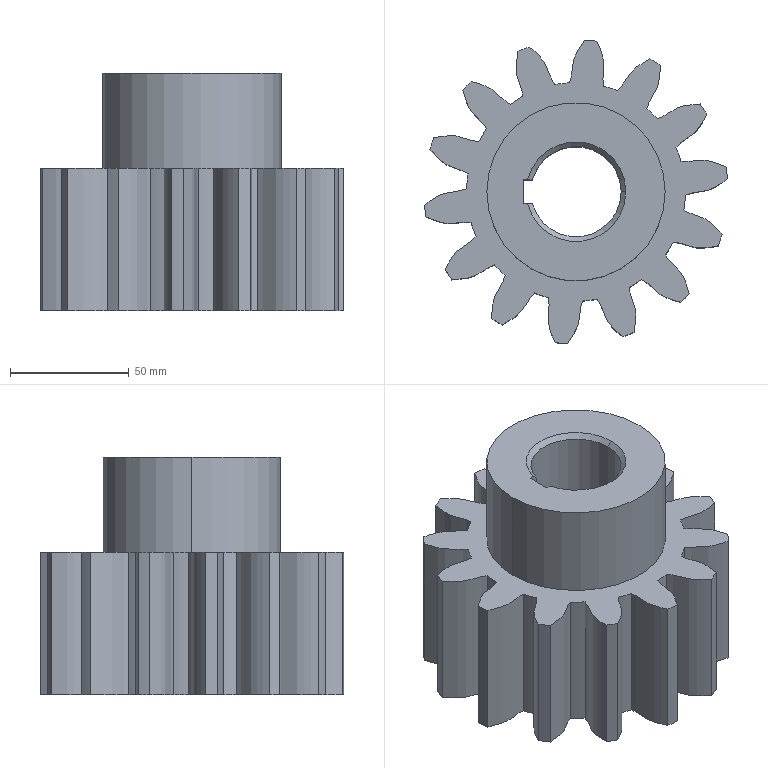Part | SolidWorks | features ICE 4, Chamfer 1, CirPattern 1, Extrusion 1 | 1 solid | 70 faces | box 127.519 x 127.793 x 100 mm | volume 607149 mm3 | cylinder 33 | spline 28 | plane 7 | cone 2 | commonest cylinder face diameters 92 x14 128 x14 55 x2 75 x2 38 x1